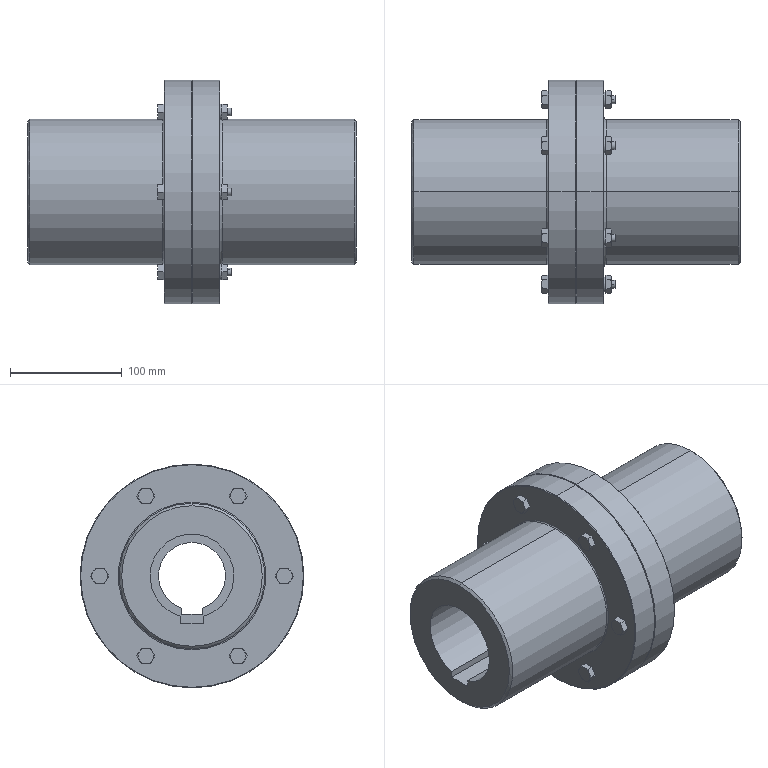Part | SolidWorks | features ICE 15, Chamfer 6, Revolution 3, CirPattern 2, Fillet 2 | 1 solid | 323 faces | box 294 x 200 x 200 mm | volume 3610457 mm3 | cone 144 | plane 114 | cylinder 61 | torus 4 | commonest cylinder face diameters 7 x36 14 x12 130 x4 200 x4 60 x2 140 x2